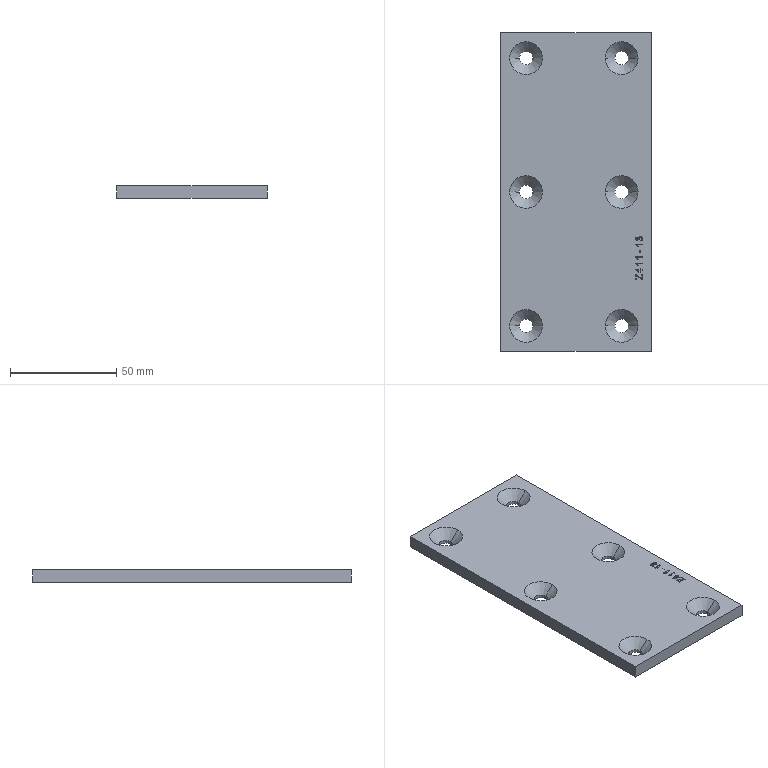Part | Creo | 1 solid | 125 faces | box 71 x 150 x 6 mm | volume 60927 mm3 | plane 53 | other 47 | cylinder 13 | cone 12 | commonest cylinder face diameters 6.4 x12 45.582 x1